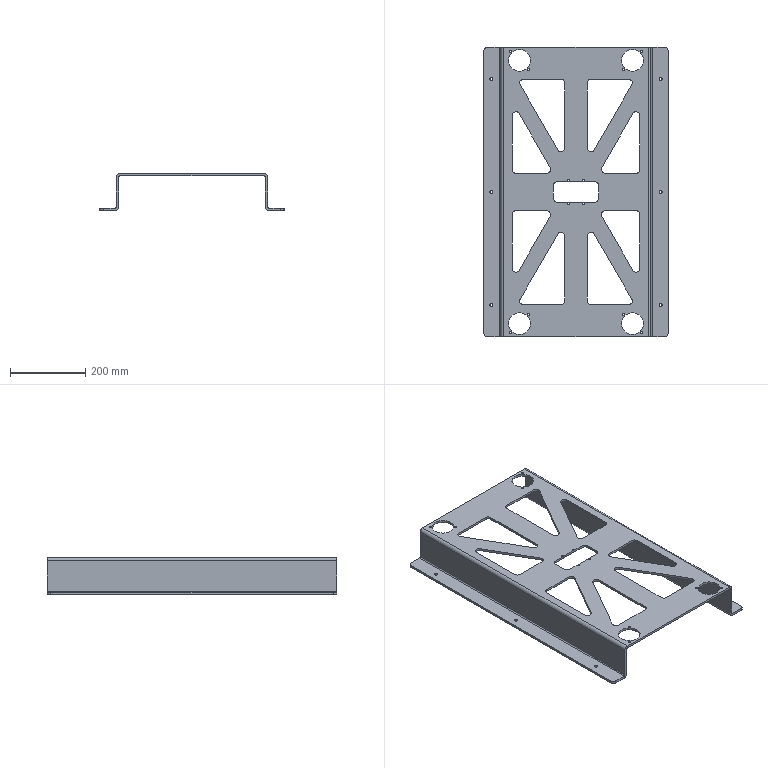Part | STEP file | LOWER.BRACKET.2.stp | 1 solid | 134 faces | box 490 x 770 x 98 mm | volume 2389480 mm3 | spline 61 | cylinder 50 | plane 23 | commonest cylinder face diameters 20 x20 6 x12 8 x6 5 x4 18 x4 58 x4